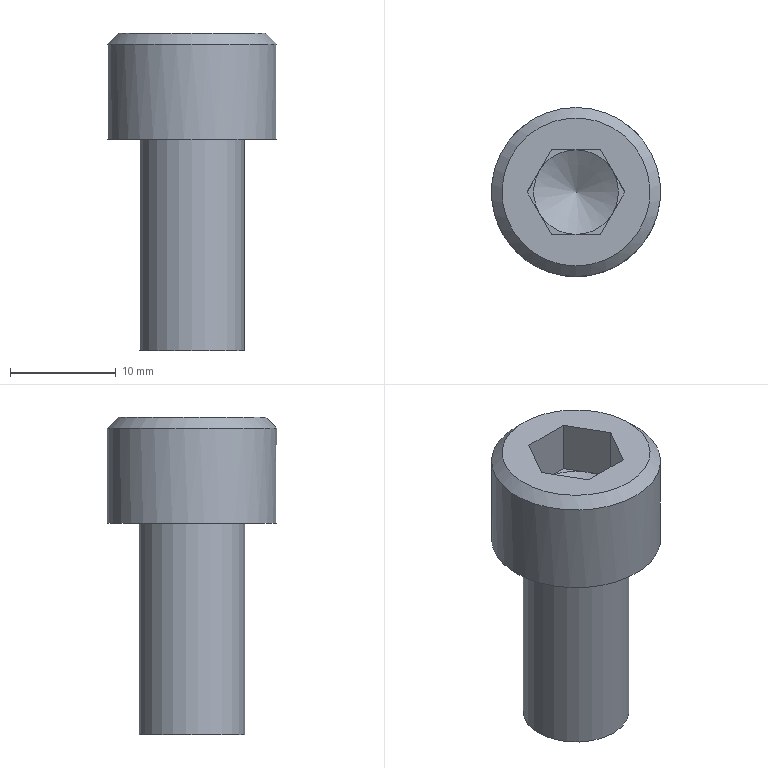Part | NX | features 5003_318_CB10-20 2 | 1 solid | 19 faces | box 16 x 16 x 30 mm | volume 3240 mm3 | plane 15 | cylinder 2 | cone 2 | commonest cylinder face diameters 10 x1 16 x1
STEP:
#1=CARTESIAN_POINT('',(258.525,-44.,-157.5));
#2=VERTEX_POINT('',#1);
#3=CARTESIAN_POINT('',(258.525,-37.,-157.5));
#4=DIRECTION('',(0.,0.,-1.));
#5=DIRECTION('',(0.,-1.,0.));
#6=AXIS2_PLACEMENT_3D('',#3,#4,#5);
#7=CIRCLE('',#6,7.);
#8=EDGE_CURVE('',#2,#2,#7,.F.);
#9=ORIENTED_EDGE('',*,*,#8,.T.);
#10=EDGE_LOOP('',(#9));
#11=FACE_BOUND('',#10,.T.);
#12=CARTESIAN_POINT('',(263.144,-37.,-157.5));
#13=VERTEX_POINT('',#12);
#14=CARTESIAN_POINT('',(260.834,-33.,-157.5));
#15=VERTEX_POINT('',#14);
#16=CARTESIAN_POINT('',(263.144,-37.,-157.5));
#17=DIRECTION('',(-0.5,0.866,0.));
#18=VECTOR('',#17,1000.);
#19=LINE('',#16,#18);
#20=EDGE_CURVE('',#13,#15,#19,.T.);
#21=ORIENTED_EDGE('',*,*,#20,.F.);
#22=CARTESIAN_POINT('',(260.834,-41.,-157.5));
#23=VERTEX_POINT('',#22);
#24=CARTESIAN_POINT('',(260.834,-41.,-157.5));
#25=DIRECTION('',(0.5,0.866,0.));
#26=VECTOR('',#25,1000.);
#27=LINE('',#24,#26);
#28=EDGE_CURVE('',#23,#13,#27,.T.);
#29=ORIENTED_EDGE('',*,*,#28,.F.);
#30=CARTESIAN_POINT('',(256.216,-41.,-157.5));
#31=VERTEX_POINT('',#30);
#32=CARTESIAN_POINT('',(256.216,-41.,-157.5));
#33=DIRECTION('',(1.,0.,0.));
#34=VECTOR('',#33,1000.);
#35=LINE('',#32,#34);
#36=EDGE_CURVE('',#31,#23,#35,.T.);
#37=ORIENTED_EDGE('',*,*,#36,.F.);
#38=CARTESIAN_POINT('',(253.906,-37.,-157.5));
#39=VERTEX_POINT('',#38);
#40=CARTESIAN_POINT('',(253.906,-37.,-157.5));
#41=DIRECTION('',(0.5,-0.866,0.));
#42=VECTOR('',#41,1000.);
#43=LINE('',#40,#42);
#44=EDGE_CURVE('',#39,#31,#43,.T.);
#45=ORIENTED_EDGE('',*,*,#44,.F.);
#46=CARTESIAN_POINT('',(256.216,-33.,-157.5));
#47=VERTEX_POINT('',#46);
#48=CARTESIAN_POINT('',(256.216,-33.,-157.5));
#49=DIRECTION('',(-0.5,-0.866,0.));
#50=VECTOR('',#49,1000.);
#51=LINE('',#48,#50);
#52=EDGE_CURVE('',#47,#39,#51,.T.);
#53=ORIENTED_EDGE('',*,*,#52,.F.);
#54=CARTESIAN_POINT('',(260.834,-33.,-157.5));
#55=DIRECTION('',(-1.,0.,0.));
#56=VECTOR('',#55,1000.);
#57=LINE('',#54,#56);
#58=EDGE_CURVE('',#15,#47,#57,.T.);
#59=ORIENTED_EDGE('',*,*,#58,.F.);
#60=EDGE_LOOP('',(#21,#29,#37,#45,#53,#59));
#61=FACE_BOUND('',#60,.T.);
#62=CARTESIAN_POINT('',(250.525,-37.,-157.5));
#63=DIRECTION('',(0.,0.,-1.));
#64=DIRECTION('',(0.,-1.,0.));
#65=AXIS2_PLACEMENT_3D('',#62,#63,#64);
#66=PLANE('',#65);
#67=ADVANCED_FACE('',(#11,#61),#66,.F.);
#68=CARTESIAN_POINT('',(258.525,-32.,-187.5));
#69=VERTEX_POINT('',#68);
#70=CARTESIAN_POINT('',(258.525,-37.,-187.5));
#71=DIRECTION('',(0.,0.,1.));
#72=DIRECTION('',(0.,1.,0.));
#73=AXIS2_PLACEMENT_3D('',#70,#71,#72);
#74=CIRCLE('',#73,5.);
#75=EDGE_CURVE('',#69,#69,#74,.T.);
#76=ORIENTED_EDGE('',*,*,#75,.F.);
#77=EDGE_LOOP('',(#76));
#78=FACE_BOUND('',#77,.T.);
#79=CARTESIAN_POINT('',(258.525,-37.,-187.5));
#80=DIRECTION('',(0.,0.,1.));
#81=DIRECTION('',(0.,1.,0.));
#82=AXIS2_PLACEMENT_3D('',#79,#80,#81);
#83=PLANE('',#82);
#84=ADVANCED_FACE('',(#78),#83,.F.);
#85=CARTESIAN_POINT('',(258.525,-32.,-167.5));
#86=VERTEX_POINT('',#85);
#87=CARTESIAN_POINT('',(258.525,-37.,-167.5));
#88=DIRECTION('',(0.,0.,1.));
#89=DIRECTION('',(0.,1.,0.));
#90=AXIS2_PLACEMENT_3D('',#87,#88,#89);
#91=CIRCLE('',#90,5.);
#92=EDGE_CURVE('',#86,#86,#91,.T.);
#93=ORIENTED_EDGE('',*,*,#92,.F.);
#94=EDGE_LOOP('',(#93));
#95=FACE_BOUND('',#94,.T.);
#96=ORIENTED_EDGE('',*,*,#75,.T.);
#97=EDGE_LOOP('',(#96));
#98=FACE_BOUND('',#97,.T.);
#99=CARTESIAN_POINT('',(258.525,-37.,-157.5));
#100=DIRECTION('',(0.,0.,1.));
#101=DIRECTION('',(0.,1.,0.));
#102=AXIS2_PLACEMENT_3D('',#99,#100,#101);
#103=CYLINDRICAL_SURFACE('',#102,5.);
#104=ADVANCED_FACE('',(#95,#98),#103,.T.);
#105=CARTESIAN_POINT('',(258.525,-29.,-167.5));
#106=VERTEX_POINT('',#105);
#107=CARTESIAN_POINT('',(258.525,-37.,-167.5));
#108=DIRECTION('',(0.,0.,1.));
#109=DIRECTION('',(0.,1.,0.));
#110=AXIS2_PLACEMENT_3D('',#107,#108,#109);
#111=CIRCLE('',#110,8.);
#112=EDGE_CURVE('',#106,#106,#111,.T.);
#113=ORIENTED_EDGE('',*,*,#112,.F.);
#114=EDGE_LOOP('',(#113));
#115=FACE_BOUND('',#114,.T.);
#116=ORIENTED_EDGE('',*,*,#92,.T.);
#117=EDGE_LOOP('',(#116));
#118=FACE_BOUND('',#117,.T.);
#119=CARTESIAN_POINT('',(253.525,-37.,-167.5));
#120=DIRECTION('',(0.,0.,1.));
#121=DIRECTION('',(0.,1.,0.));
#122=AXIS2_PLACEMENT_3D('',#119,#120,#121);
#123=PLANE('',#122);
#124=ADVANCED_FACE('',(#115,#118),#123,.F.);
#125=CARTESIAN_POINT('',(258.525,-45.,-158.5));
#126=VERTEX_POINT('',#125);
#127=CARTESIAN_POINT('',(258.525,-37.,-158.5));
#128=DIRECTION('',(0.,0.,-1.));
#129=DIRECTION('',(0.,-1.,0.));
#130=AXIS2_PLACEMENT_3D('',#127,#128,#129);
#131=CIRCLE('',#130,8.);
#132=EDGE_CURVE('',#126,#126,#131,.T.);
#133=ORIENTED_EDGE('',*,*,#132,.T.);
#134=EDGE_LOOP('',(#133));
#135=FACE_BOUND('',#134,.T.);
#136=ORIENTED_EDGE('',*,*,#112,.T.);
#137=EDGE_LOOP('',(#136));
#138=FACE_BOUND('',#137,.T.);
#139=CARTESIAN_POINT('',(258.525,-37.,-157.5));
#140=DIRECTION('',(0.,0.,1.));
#141=DIRECTION('',(0.,1.,0.));
#142=AXIS2_PLACEMENT_3D('',#139,#140,#141);
#143=CYLINDRICAL_SURFACE('',#142,8.);
#144=ADVANCED_FACE('',(#135,#138),#143,.T.);
#145=ORIENTED_EDGE('',*,*,#132,.F.);
#146=EDGE_LOOP('',(#145));
#147=FACE_BOUND('',#146,.T.);
#148=ORIENTED_EDGE('',*,*,#8,.F.);
#149=EDGE_LOOP('',(#148));
#150=FACE_BOUND('',#149,.T.);
#151=CARTESIAN_POINT('',(258.525,-37.,-157.5));
#152=DIRECTION('',(0.,0.,-1.));
#153=DIRECTION('',(0.,-1.,0.));
#154=AXIS2_PLACEMENT_3D('',#151,#152,#153);
#155=CONICAL_SURFACE('',#154,7.,0.7854);
#156=ADVANCED_FACE('',(#147,#150),#155,.T.);
#157=CARTESIAN_POINT('',(260.834,-41.,-162.5));
#158=VERTEX_POINT('',#157);
#159=CARTESIAN_POINT('',(261.989,-39.,-162.5));
#160=VERTEX_POINT('',#159);
#161=CARTESIAN_POINT('',(260.834,-41.,-162.5));
#162=DIRECTION('',(0.5,0.866,0.));
#163=VECTOR('',#162,1000.);
#164=LINE('',#161,#163);
#165=EDGE_CURVE('',#158,#160,#164,.T.);
#166=ORIENTED_EDGE('',*,*,#165,.F.);
#167=CARTESIAN_POINT('',(260.834,-41.,-162.5));
#168=DIRECTION('',(0.,0.,1.));
#169=VECTOR('',#168,1000.);
#170=LINE('',#167,#169);
#171=EDGE_CURVE('',#158,#23,#170,.T.);
#172=ORIENTED_EDGE('',*,*,#171,.T.);
#173=ORIENTED_EDGE('',*,*,#28,.T.);
#174=CARTESIAN_POINT('',(263.144,-37.,-162.5));
#175=VERTEX_POINT('',#174);
#176=CARTESIAN_POINT('',(263.144,-37.,-162.5));
#177=DIRECTION('',(0.,0.,1.));
#178=VECTOR('',#177,1000.);
#179=LINE('',#176,#178);
#180=EDGE_CURVE('',#175,#13,#179,.T.);
#181=ORIENTED_EDGE('',*,*,#180,.F.);
#182=CARTESIAN_POINT('',(260.834,-41.,-162.5));
#183=DIRECTION('',(0.5,0.866,0.));
#184=VECTOR('',#183,1000.);
#185=LINE('',#182,#184);
#186=EDGE_CURVE('',#160,#175,#185,.T.);
#187=ORIENTED_EDGE('',*,*,#186,.F.);
#188=EDGE_LOOP('',(#166,#172,#173,#181,#187));
#189=FACE_BOUND('',#188,.T.);
#190=CARTESIAN_POINT('',(260.834,-41.,-162.5));
#191=DIRECTION('',(0.866,-0.5,0.));
#192=DIRECTION('',(-0.5,-0.866,0.));
#193=AXIS2_PLACEMENT_3D('',#190,#191,#192);
#194=PLANE('',#193);
#195=ADVANCED_FACE('',(#189),#194,.F.);
#196=CARTESIAN_POINT('',(256.216,-41.,-162.5));
#197=VERTEX_POINT('',#196);
#198=CARTESIAN_POINT('',(258.525,-41.,-162.5));
#199=VERTEX_POINT('',#198);
#200=CARTESIAN_POINT('',(256.216,-41.,-162.5));
#201=DIRECTION('',(1.,0.,0.));
#202=VECTOR('',#201,1000.);
#203=LINE('',#200,#202);
#204=EDGE_CURVE('',#197,#199,#203,.T.);
#205=ORIENTED_EDGE('',*,*,#204,.F.);
#206=CARTESIAN_POINT('',(256.216,-41.,-162.5));
#207=DIRECTION('',(0.,0.,1.));
#208=VECTOR('',#207,1000.);
#209=LINE('',#206,#208);
#210=EDGE_CURVE('',#197,#31,#209,.T.);
#211=ORIENTED_EDGE('',*,*,#210,.T.);
#212=ORIENTED_EDGE('',*,*,#36,.T.);
#213=ORIENTED_EDGE('',*,*,#171,.F.);
#214=CARTESIAN_POINT('',(256.216,-41.,-162.5));
#215=DIRECTION('',(1.,0.,0.));
#216=VECTOR('',#215,1000.);
#217=LINE('',#214,#216);
#218=EDGE_CURVE('',#199,#158,#217,.T.);
#219=ORIENTED_EDGE('',*,*,#218,.F.);
#220=EDGE_LOOP('',(#205,#211,#212,#213,#219));
#221=FACE_BOUND('',#220,.T.);
#222=CARTESIAN_POINT('',(256.216,-41.,-162.5));
#223=DIRECTION('',(0.,-1.,0.));
#224=DIRECTION('',(0.,0.,1.));
#225=AXIS2_PLACEMENT_3D('',#222,#223,#224);
#226=PLANE('',#225);
#227=ADVANCED_FACE('',(#221),#226,.F.);
#228=CARTESIAN_POINT('',(253.906,-37.,-162.5));
#229=VERTEX_POINT('',#228);
#230=CARTESIAN_POINT('',(255.061,-39.,-162.5));
#231=VERTEX_POINT('',#230);
#232=CARTESIAN_POINT('',(253.906,-37.,-162.5));
#233=DIRECTION('',(0.5,-0.866,0.));
#234=VECTOR('',#233,1000.);
#235=LINE('',#232,#234);
#236=EDGE_CURVE('',#229,#231,#235,.T.);
#237=ORIENTED_EDGE('',*,*,#236,.F.);
#238=CARTESIAN_POINT('',(253.906,-37.,-162.5));
#239=DIRECTION('',(0.,0.,1.));
#240=VECTOR('',#239,1000.);
#241=LINE('',#238,#240);
#242=EDGE_CURVE('',#229,#39,#241,.T.);
#243=ORIENTED_EDGE('',*,*,#242,.T.);
#244=ORIENTED_EDGE('',*,*,#44,.T.);
#245=ORIENTED_EDGE('',*,*,#210,.F.);
#246=CARTESIAN_POINT('',(253.906,-37.,-162.5));
#247=DIRECTION('',(0.5,-0.866,0.));
#248=VECTOR('',#247,1000.);
#249=LINE('',#246,#248);
#250=EDGE_CURVE('',#231,#197,#249,.T.);
#251=ORIENTED_EDGE('',*,*,#250,.F.);
#252=EDGE_LOOP('',(#237,#243,#244,#245,#251));
#253=FACE_BOUND('',#252,.T.);
#254=CARTESIAN_POINT('',(253.906,-37.,-162.5));
#255=DIRECTION('',(-0.866,-0.5,0.));
#256=DIRECTION('',(-0.5,0.866,0.));
#257=AXIS2_PLACEMENT_3D('',#254,#255,#256);
#258=PLANE('',#257);
#259=ADVANCED_FACE('',(#253),#258,.F.);
#260=CARTESIAN_POINT('',(256.216,-33.,-162.5));
#261=VERTEX_POINT('',#260);
#262=CARTESIAN_POINT('',(255.061,-35.,-162.5));
#263=VERTEX_POINT('',#262);
#264=CARTESIAN_POINT('',(256.216,-33.,-162.5));
#265=DIRECTION('',(-0.5,-0.866,0.));
#266=VECTOR('',#265,1000.);
#267=LINE('',#264,#266);
#268=EDGE_CURVE('',#261,#263,#267,.T.);
#269=ORIENTED_EDGE('',*,*,#268,.F.);
#270=CARTESIAN_POINT('',(256.216,-33.,-162.5));
#271=DIRECTION('',(0.,0.,1.));
#272=VECTOR('',#271,1000.);
#273=LINE('',#270,#272);
#274=EDGE_CURVE('',#261,#47,#273,.T.);
#275=ORIENTED_EDGE('',*,*,#274,.T.);
#276=ORIENTED_EDGE('',*,*,#52,.T.);
#277=ORIENTED_EDGE('',*,*,#242,.F.);
#278=CARTESIAN_POINT('',(256.216,-33.,-162.5));
#279=DIRECTION('',(-0.5,-0.866,0.));
#280=VECTOR('',#279,1000.);
#281=LINE('',#278,#280);
#282=EDGE_CURVE('',#263,#229,#281,.T.);
#283=ORIENTED_EDGE('',*,*,#282,.F.);
#284=EDGE_LOOP('',(#269,#275,#276,#277,#283));
#285=FACE_BOUND('',#284,.T.);
#286=CARTESIAN_POINT('',(256.216,-33.,-162.5));
#287=DIRECTION('',(-0.866,0.5,0.));
#288=DIRECTION('',(0.5,0.866,0.));
#289=AXIS2_PLACEMENT_3D('',#286,#287,#288);
#290=PLANE('',#289);
#291=ADVANCED_FACE('',(#285),#290,.F.);
#292=CARTESIAN_POINT('',(260.834,-33.,-162.5));
#293=VERTEX_POINT('',#292);
#294=CARTESIAN_POINT('',(258.525,-33.,-162.5));
#295=VERTEX_POINT('',#294);
#296=CARTESIAN_POINT('',(260.834,-33.,-162.5));
#297=DIRECTION('',(-1.,0.,0.));
#298=VECTOR('',#297,1000.);
#299=LINE('',#296,#298);
#300=EDGE_CURVE('',#293,#295,#299,.T.);
#301=ORIENTED_EDGE('',*,*,#300,.F.);
#302=CARTESIAN_POINT('',(260.834,-33.,-162.5));
#303=DIRECTION('',(0.,0.,1.));
#304=VECTOR('',#303,1000.);
#305=LINE('',#302,#304);
#306=EDGE_CURVE('',#293,#15,#305,.T.);
#307=ORIENTED_EDGE('',*,*,#306,.T.);
#308=ORIENTED_EDGE('',*,*,#58,.T.);
#309=ORIENTED_EDGE('',*,*,#274,.F.);
#310=CARTESIAN_POINT('',(260.834,-33.,-162.5));
#311=DIRECTION('',(-1.,0.,0.));
#312=VECTOR('',#311,1000.);
#313=LINE('',#310,#312);
#314=EDGE_CURVE('',#295,#261,#313,.T.);
#315=ORIENTED_EDGE('',*,*,#314,.F.);
#316=EDGE_LOOP('',(#301,#307,#308,#309,#315));
#317=FACE_BOUND('',#316,.T.);
#318=CARTESIAN_POINT('',(260.834,-33.,-162.5));
#319=DIRECTION('',(0.,1.,0.));
#320=DIRECTION('',(0.,0.,-1.));
#321=AXIS2_PLACEMENT_3D('',#318,#319,#320);
#322=PLANE('',#321);
#323=ADVANCED_FACE('',(#317),#322,.F.);
#324=CARTESIAN_POINT('',(261.989,-35.,-162.5));
#325=VERTEX_POINT('',#324);
#326=CARTESIAN_POINT('',(263.144,-37.,-162.5));
#327=DIRECTION('',(-0.5,0.866,0.));
#328=VECTOR('',#327,1000.);
#329=LINE('',#326,#328);
#330=EDGE_CURVE('',#175,#325,#329,.T.);
#331=ORIENTED_EDGE('',*,*,#330,.F.);
#332=ORIENTED_EDGE('',*,*,#180,.T.);
#333=ORIENTED_EDGE('',*,*,#20,.T.);
#334=ORIENTED_EDGE('',*,*,#306,.F.);
#335=CARTESIAN_POINT('',(263.144,-37.,-162.5));
#336=DIRECTION('',(-0.5,0.866,0.));
#337=VECTOR('',#336,1000.);
#338=LINE('',#335,#337);
#339=EDGE_CURVE('',#325,#293,#338,.T.);
#340=ORIENTED_EDGE('',*,*,#339,.F.);
#341=EDGE_LOOP('',(#331,#332,#333,#334,#340));
#342=FACE_BOUND('',#341,.T.);
#343=CARTESIAN_POINT('',(263.144,-37.,-162.5));
#344=DIRECTION('',(0.866,0.5,0.));
#345=DIRECTION('',(0.5,-0.866,0.));
#346=AXIS2_PLACEMENT_3D('',#343,#344,#345);
#347=PLANE('',#346);
#348=ADVANCED_FACE('',(#342),#347,.F.);
#349=ORIENTED_EDGE('',*,*,#314,.T.);
#350=ORIENTED_EDGE('',*,*,#268,.T.);
#351=CARTESIAN_POINT('',(258.525,-37.,-162.5));
#352=DIRECTION('',(0.,0.,1.));
#353=DIRECTION('',(1.,0.,0.));
#354=AXIS2_PLACEMENT_3D('',#351,#352,#353);
#355=CIRCLE('',#354,4.);
#356=EDGE_CURVE('',#295,#263,#355,.T.);
#357=ORIENTED_EDGE('',*,*,#356,.F.);
#358=EDGE_LOOP('',(#349,#350,#357));
#359=FACE_BOUND('',#358,.T.);
#360=CARTESIAN_POINT('',(258.525,-37.,-162.5));
#361=DIRECTION('',(0.,0.,1.));
#362=DIRECTION('',(0.,1.,0.));
#363=AXIS2_PLACEMENT_3D('',#360,#361,#362);
#364=PLANE('',#363);
#365=ADVANCED_FACE('',(#359),#364,.T.);
#366=ORIENTED_EDGE('',*,*,#282,.T.);
#367=ORIENTED_EDGE('',*,*,#236,.T.);
#368=CARTESIAN_POINT('',(258.525,-37.,-162.5));
#369=DIRECTION('',(0.,0.,1.));
#370=DIRECTION('',(1.,0.,0.));
#371=AXIS2_PLACEMENT_3D('',#368,#369,#370);
#372=CIRCLE('',#371,4.);
#373=EDGE_CURVE('',#263,#231,#372,.T.);
#374=ORIENTED_EDGE('',*,*,#373,.F.);
#375=EDGE_LOOP('',(#366,#367,#374));
#376=FACE_BOUND('',#375,.T.);
#377=CARTESIAN_POINT('',(258.525,-37.,-162.5));
#378=DIRECTION('',(0.,0.,1.));
#379=DIRECTION('',(0.,1.,0.));
#380=AXIS2_PLACEMENT_3D('',#377,#378,#379);
#381=PLANE('',#380);
#382=ADVANCED_FACE('',(#376),#381,.T.);
#383=ORIENTED_EDGE('',*,*,#250,.T.);
#384=ORIENTED_EDGE('',*,*,#204,.T.);
#385=CARTESIAN_POINT('',(258.525,-37.,-162.5));
#386=DIRECTION('',(0.,0.,1.));
#387=DIRECTION('',(1.,0.,0.));
#388=AXIS2_PLACEMENT_3D('',#385,#386,#387);
#389=CIRCLE('',#388,4.);
#390=EDGE_CURVE('',#231,#199,#389,.T.);
#391=ORIENTED_EDGE('',*,*,#390,.F.);
#392=EDGE_LOOP('',(#383,#384,#391));
#393=FACE_BOUND('',#392,.T.);
#394=CARTESIAN_POINT('',(258.525,-37.,-162.5));
#395=DIRECTION('',(0.,0.,1.));
#396=DIRECTION('',(0.,1.,0.));
#397=AXIS2_PLACEMENT_3D('',#394,#395,#396);
#398=PLANE('',#397);
#399=ADVANCED_FACE('',(#393),#398,.T.);
#400=ORIENTED_EDGE('',*,*,#218,.T.);
#401=ORIENTED_EDGE('',*,*,#165,.T.);
#402=CARTESIAN_POINT('',(258.525,-37.,-162.5));
#403=DIRECTION('',(0.,0.,1.));
#404=DIRECTION('',(1.,0.,0.));
#405=AXIS2_PLACEMENT_3D('',#402,#403,#404);
#406=CIRCLE('',#405,4.);
#407=EDGE_CURVE('',#199,#160,#406,.T.);
#408=ORIENTED_EDGE('',*,*,#407,.F.);
#409=EDGE_LOOP('',(#400,#401,#408));
#410=FACE_BOUND('',#409,.T.);
#411=CARTESIAN_POINT('',(258.525,-37.,-162.5));
#412=DIRECTION('',(0.,0.,1.));
#413=DIRECTION('',(0.,1.,0.));
#414=AXIS2_PLACEMENT_3D('',#411,#412,#413);
#415=PLANE('',#414);
#416=ADVANCED_FACE('',(#410),#415,.T.);
#417=ORIENTED_EDGE('',*,*,#186,.T.);
#418=ORIENTED_EDGE('',*,*,#330,.T.);
#419=CARTESIAN_POINT('',(258.525,-37.,-162.5));
#420=DIRECTION('',(0.,0.,1.));
#421=DIRECTION('',(1.,0.,0.));
#422=AXIS2_PLACEMENT_3D('',#419,#420,#421);
#423=CIRCLE('',#422,4.);
#424=EDGE_CURVE('',#160,#325,#423,.T.);
#425=ORIENTED_EDGE('',*,*,#424,.F.);
#426=EDGE_LOOP('',(#417,#418,#425));
#427=FACE_BOUND('',#426,.T.);
#428=CARTESIAN_POINT('',(258.525,-37.,-162.5));
#429=DIRECTION('',(0.,0.,1.));
#430=DIRECTION('',(0.,1.,0.));
#431=AXIS2_PLACEMENT_3D('',#428,#429,#430);
#432=PLANE('',#431);
#433=ADVANCED_FACE('',(#427),#432,.T.);
#434=ORIENTED_EDGE('',*,*,#339,.T.);
#435=ORIENTED_EDGE('',*,*,#300,.T.);
#436=CARTESIAN_POINT('',(258.525,-37.,-162.5));
#437=DIRECTION('',(0.,0.,1.));
#438=DIRECTION('',(1.,0.,0.));
#439=AXIS2_PLACEMENT_3D('',#436,#437,#438);
#440=CIRCLE('',#439,4.);
#441=EDGE_CURVE('',#325,#295,#440,.T.);
#442=ORIENTED_EDGE('',*,*,#441,.F.);
#443=EDGE_LOOP('',(#434,#435,#442));
#444=FACE_BOUND('',#443,.T.);
#445=CARTESIAN_POINT('',(258.525,-37.,-162.5));
#446=DIRECTION('',(0.,0.,1.));
#447=DIRECTION('',(0.,1.,0.));
#448=AXIS2_PLACEMENT_3D('',#445,#446,#447);
#449=PLANE('',#448);
#450=ADVANCED_FACE('',(#444),#449,.T.);
#451=ORIENTED_EDGE('',*,*,#441,.T.);
#452=ORIENTED_EDGE('',*,*,#356,.T.);
#453=ORIENTED_EDGE('',*,*,#373,.T.);
#454=ORIENTED_EDGE('',*,*,#390,.T.);
#455=ORIENTED_EDGE('',*,*,#407,.T.);
#456=ORIENTED_EDGE('',*,*,#424,.T.);
#457=EDGE_LOOP('',(#451,#452,#453,#454,#455,#456));
#458=FACE_BOUND('',#457,.T.);
#459=CARTESIAN_POINT('',(258.525,-37.,-164.903));
#460=VERTEX_POINT('',#459);
#461=VERTEX_LOOP('',#460);
#462=FACE_BOUND('',#461,.T.);
#463=CARTESIAN_POINT('',(258.525,-37.,-164.903));
#464=DIRECTION('',(0.,0.,1.));
#465=DIRECTION('',(1.,0.,0.));
#466=AXIS2_PLACEMENT_3D('',#463,#464,#465);
#467=CONICAL_SURFACE('',#466,0.,1.03);
#468=ADVANCED_FACE('',(#458,#462),#467,.F.);
#469=CLOSED_SHELL('',(#67,#84,#104,#124,#144,#156,#195,#227,#259,#291,#323,#348,#365,#382,#399,#416,#433,#450,#468));
#470=MANIFOLD_SOLID_BREP('',#469);
#471=(LENGTH_UNIT()NAMED_UNIT(*)SI_UNIT(.MILLI.,.METRE.));
#472=UNCERTAINTY_MEASURE_WITH_UNIT(LENGTH_MEASURE(0.00001),#471,'','');
#473=(NAMED_UNIT(*)PLANE_ANGLE_UNIT()SI_UNIT($,.RADIAN.));
#474=(NAMED_UNIT(*)SI_UNIT($,.STERADIAN.)SOLID_ANGLE_UNIT());
#475=(GEOMETRIC_REPRESENTATION_CONTEXT(3)GLOBAL_UNCERTAINTY_ASSIGNED_CONTEXT((#472))GLOBAL_UNIT_ASSIGNED_CONTEXT((#471,#473,#474))REPRESENTATION_CONTEXT('',''));
#476=ADVANCED_BREP_SHAPE_REPRESENTATION('',(#470),#475);